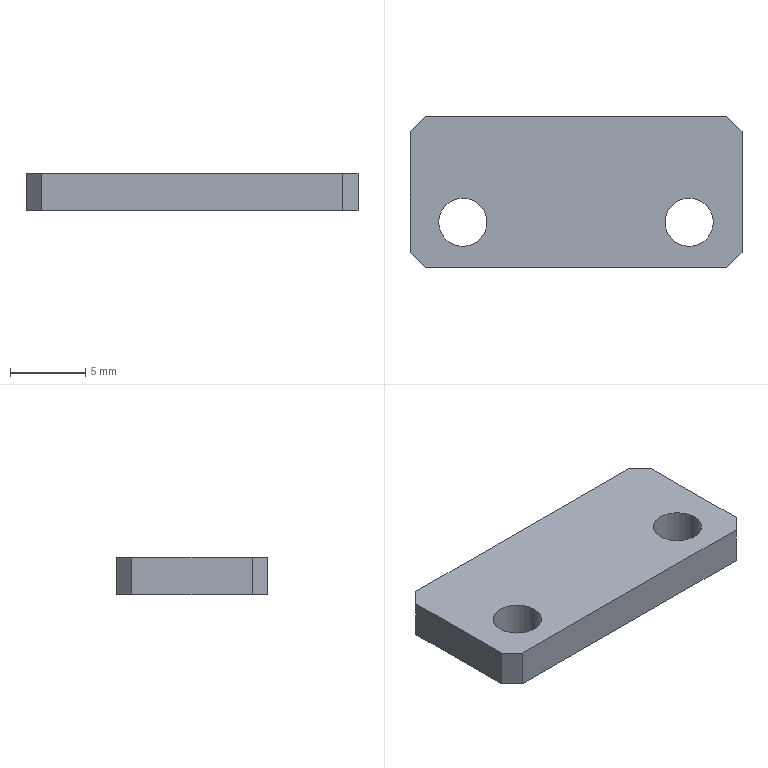Part | NX | features BREP 1 | 1 solid | 14 faces | box 22 x 10 x 2.5 mm | volume 504.788 mm3 | plane 10 | cylinder 4 | commonest cylinder face diameters 3.2 x4
STEP:
#1=CARTESIAN_POINT('',(-697.082,-312.703,0.));
#2=VERTEX_POINT('',#1);
#3=CARTESIAN_POINT('',(-693.882,-312.703,0.));
#4=VERTEX_POINT('',#3);
#5=CARTESIAN_POINT('',(-695.482,-312.703,0.));
#6=DIRECTION('',(0.,0.,1.));
#7=DIRECTION('',(1.,0.,0.));
#8=AXIS2_PLACEMENT_3D('',#5,#6,#7);
#9=CIRCLE('',#8,1.6);
#10=EDGE_CURVE('',#2,#4,#9,.T.);
#11=ORIENTED_EDGE('',*,*,#10,.F.);
#12=CARTESIAN_POINT('',(-697.082,-312.703,2.5));
#13=VERTEX_POINT('',#12);
#14=CARTESIAN_POINT('',(-697.082,-312.703,0.));
#15=DIRECTION('',(0.,0.,1.));
#16=VECTOR('',#15,1000.);
#17=LINE('',#14,#16);
#18=EDGE_CURVE('',#13,#2,#17,.F.);
#19=ORIENTED_EDGE('',*,*,#18,.F.);
#20=CARTESIAN_POINT('',(-693.882,-312.703,2.5));
#21=VERTEX_POINT('',#20);
#22=CARTESIAN_POINT('',(-695.482,-312.703,2.5));
#23=DIRECTION('',(0.,0.,1.));
#24=DIRECTION('',(1.,0.,0.));
#25=AXIS2_PLACEMENT_3D('',#22,#23,#24);
#26=CIRCLE('',#25,1.6);
#27=EDGE_CURVE('',#13,#21,#26,.T.);
#28=ORIENTED_EDGE('',*,*,#27,.T.);
#29=CARTESIAN_POINT('',(-693.882,-312.703,0.));
#30=DIRECTION('',(0.,0.,1.));
#31=VECTOR('',#30,1000.);
#32=LINE('',#29,#31);
#33=EDGE_CURVE('',#21,#4,#32,.F.);
#34=ORIENTED_EDGE('',*,*,#33,.T.);
#35=EDGE_LOOP('',(#11,#19,#28,#34));
#36=FACE_BOUND('',#35,.T.);
#37=CARTESIAN_POINT('',(-695.482,-312.703,0.));
#38=DIRECTION('',(0.,0.,1.));
#39=DIRECTION('',(1.,0.,0.));
#40=AXIS2_PLACEMENT_3D('',#37,#38,#39);
#41=CYLINDRICAL_SURFACE('',#40,1.6);
#42=ADVANCED_FACE('',(#36),#41,.F.);
#43=CARTESIAN_POINT('',(-712.082,-312.703,0.));
#44=VERTEX_POINT('',#43);
#45=CARTESIAN_POINT('',(-708.882,-312.703,0.));
#46=VERTEX_POINT('',#45);
#47=CARTESIAN_POINT('',(-710.482,-312.703,0.));
#48=DIRECTION('',(0.,0.,1.));
#49=DIRECTION('',(1.,0.,0.));
#50=AXIS2_PLACEMENT_3D('',#47,#48,#49);
#51=CIRCLE('',#50,1.6);
#52=EDGE_CURVE('',#44,#46,#51,.T.);
#53=ORIENTED_EDGE('',*,*,#52,.F.);
#54=CARTESIAN_POINT('',(-712.082,-312.703,2.5));
#55=VERTEX_POINT('',#54);
#56=CARTESIAN_POINT('',(-712.082,-312.703,0.));
#57=DIRECTION('',(0.,0.,1.));
#58=VECTOR('',#57,1000.);
#59=LINE('',#56,#58);
#60=EDGE_CURVE('',#55,#44,#59,.F.);
#61=ORIENTED_EDGE('',*,*,#60,.F.);
#62=CARTESIAN_POINT('',(-708.882,-312.703,2.5));
#63=VERTEX_POINT('',#62);
#64=CARTESIAN_POINT('',(-710.482,-312.703,2.5));
#65=DIRECTION('',(0.,0.,1.));
#66=DIRECTION('',(1.,0.,0.));
#67=AXIS2_PLACEMENT_3D('',#64,#65,#66);
#68=CIRCLE('',#67,1.6);
#69=EDGE_CURVE('',#55,#63,#68,.T.);
#70=ORIENTED_EDGE('',*,*,#69,.T.);
#71=CARTESIAN_POINT('',(-708.882,-312.703,0.));
#72=DIRECTION('',(0.,0.,1.));
#73=VECTOR('',#72,1000.);
#74=LINE('',#71,#73);
#75=EDGE_CURVE('',#63,#46,#74,.F.);
#76=ORIENTED_EDGE('',*,*,#75,.T.);
#77=EDGE_LOOP('',(#53,#61,#70,#76));
#78=FACE_BOUND('',#77,.T.);
#79=CARTESIAN_POINT('',(-710.482,-312.703,0.));
#80=DIRECTION('',(0.,0.,1.));
#81=DIRECTION('',(1.,0.,0.));
#82=AXIS2_PLACEMENT_3D('',#79,#80,#81);
#83=CYLINDRICAL_SURFACE('',#82,1.6);
#84=ADVANCED_FACE('',(#78),#83,.F.);
#85=CARTESIAN_POINT('',(-713.982,-306.703,2.5));
#86=VERTEX_POINT('',#85);
#87=CARTESIAN_POINT('',(-713.982,-314.703,2.5));
#88=VERTEX_POINT('',#87);
#89=CARTESIAN_POINT('',(-713.982,-305.703,2.5));
#90=DIRECTION('',(0.,-1.,0.));
#91=VECTOR('',#90,1000.);
#92=LINE('',#89,#91);
#93=EDGE_CURVE('',#86,#88,#92,.T.);
#94=ORIENTED_EDGE('',*,*,#93,.F.);
#95=CARTESIAN_POINT('',(-713.982,-306.703,0.));
#96=VERTEX_POINT('',#95);
#97=CARTESIAN_POINT('',(-713.982,-306.703,2.5));
#98=DIRECTION('',(0.,0.,-1.));
#99=VECTOR('',#98,1000.);
#100=LINE('',#97,#99);
#101=EDGE_CURVE('',#86,#96,#100,.T.);
#102=ORIENTED_EDGE('',*,*,#101,.T.);
#103=CARTESIAN_POINT('',(-713.982,-314.703,0.));
#104=VERTEX_POINT('',#103);
#105=CARTESIAN_POINT('',(-713.982,-305.703,0.));
#106=DIRECTION('',(0.,-1.,0.));
#107=VECTOR('',#106,1000.);
#108=LINE('',#105,#107);
#109=EDGE_CURVE('',#96,#104,#108,.T.);
#110=ORIENTED_EDGE('',*,*,#109,.T.);
#111=CARTESIAN_POINT('',(-713.982,-314.703,2.5));
#112=DIRECTION('',(0.,0.,1.));
#113=VECTOR('',#112,1000.);
#114=LINE('',#111,#113);
#115=EDGE_CURVE('',#104,#88,#114,.T.);
#116=ORIENTED_EDGE('',*,*,#115,.T.);
#117=EDGE_LOOP('',(#94,#102,#110,#116));
#118=FACE_BOUND('',#117,.T.);
#119=CARTESIAN_POINT('',(-713.982,-305.703,2.5));
#120=DIRECTION('',(1.,0.,0.));
#121=DIRECTION('',(0.,1.,0.));
#122=AXIS2_PLACEMENT_3D('',#119,#120,#121);
#123=PLANE('',#122);
#124=ADVANCED_FACE('',(#118),#123,.F.);
#125=CARTESIAN_POINT('',(-712.982,-315.703,0.));
#126=VERTEX_POINT('',#125);
#127=CARTESIAN_POINT('',(-692.982,-315.703,0.));
#128=VERTEX_POINT('',#127);
#129=CARTESIAN_POINT('',(-713.982,-315.703,0.));
#130=DIRECTION('',(1.,0.,0.));
#131=VECTOR('',#130,1000.);
#132=LINE('',#129,#131);
#133=EDGE_CURVE('',#126,#128,#132,.T.);
#134=ORIENTED_EDGE('',*,*,#133,.T.);
#135=CARTESIAN_POINT('',(-692.982,-315.703,2.5));
#136=VERTEX_POINT('',#135);
#137=CARTESIAN_POINT('',(-692.982,-315.703,2.5));
#138=DIRECTION('',(0.,0.,1.));
#139=VECTOR('',#138,1000.);
#140=LINE('',#137,#139);
#141=EDGE_CURVE('',#128,#136,#140,.T.);
#142=ORIENTED_EDGE('',*,*,#141,.T.);
#143=CARTESIAN_POINT('',(-712.982,-315.703,2.5));
#144=VERTEX_POINT('',#143);
#145=CARTESIAN_POINT('',(-713.982,-315.703,2.5));
#146=DIRECTION('',(1.,0.,0.));
#147=VECTOR('',#146,1000.);
#148=LINE('',#145,#147);
#149=EDGE_CURVE('',#144,#136,#148,.T.);
#150=ORIENTED_EDGE('',*,*,#149,.F.);
#151=CARTESIAN_POINT('',(-712.982,-315.703,2.5));
#152=DIRECTION('',(0.,0.,-1.));
#153=VECTOR('',#152,1000.);
#154=LINE('',#151,#153);
#155=EDGE_CURVE('',#144,#126,#154,.T.);
#156=ORIENTED_EDGE('',*,*,#155,.T.);
#157=EDGE_LOOP('',(#134,#142,#150,#156));
#158=FACE_BOUND('',#157,.T.);
#159=CARTESIAN_POINT('',(-713.982,-315.703,2.5));
#160=DIRECTION('',(0.,1.,0.));
#161=DIRECTION('',(1.,0.,0.));
#162=AXIS2_PLACEMENT_3D('',#159,#160,#161);
#163=PLANE('',#162);
#164=ADVANCED_FACE('',(#158),#163,.F.);
#165=CARTESIAN_POINT('',(-691.982,-314.703,0.));
#166=VERTEX_POINT('',#165);
#167=CARTESIAN_POINT('',(-691.982,-306.703,0.));
#168=VERTEX_POINT('',#167);
#169=CARTESIAN_POINT('',(-691.982,-305.703,0.));
#170=DIRECTION('',(0.,1.,0.));
#171=VECTOR('',#170,1000.);
#172=LINE('',#169,#171);
#173=EDGE_CURVE('',#166,#168,#172,.T.);
#174=ORIENTED_EDGE('',*,*,#173,.T.);
#175=CARTESIAN_POINT('',(-691.982,-306.703,2.5));
#176=VERTEX_POINT('',#175);
#177=CARTESIAN_POINT('',(-691.982,-306.703,2.5));
#178=DIRECTION('',(0.,0.,1.));
#179=VECTOR('',#178,1000.);
#180=LINE('',#177,#179);
#181=EDGE_CURVE('',#168,#176,#180,.T.);
#182=ORIENTED_EDGE('',*,*,#181,.T.);
#183=CARTESIAN_POINT('',(-691.982,-314.703,2.5));
#184=VERTEX_POINT('',#183);
#185=CARTESIAN_POINT('',(-691.982,-305.703,2.5));
#186=DIRECTION('',(0.,1.,0.));
#187=VECTOR('',#186,1000.);
#188=LINE('',#185,#187);
#189=EDGE_CURVE('',#184,#176,#188,.T.);
#190=ORIENTED_EDGE('',*,*,#189,.F.);
#191=CARTESIAN_POINT('',(-691.982,-314.703,2.5));
#192=DIRECTION('',(0.,0.,-1.));
#193=VECTOR('',#192,1000.);
#194=LINE('',#191,#193);
#195=EDGE_CURVE('',#184,#166,#194,.T.);
#196=ORIENTED_EDGE('',*,*,#195,.T.);
#197=EDGE_LOOP('',(#174,#182,#190,#196));
#198=FACE_BOUND('',#197,.T.);
#199=CARTESIAN_POINT('',(-691.982,-305.703,2.5));
#200=DIRECTION('',(-1.,0.,0.));
#201=DIRECTION('',(0.,0.,1.));
#202=AXIS2_PLACEMENT_3D('',#199,#200,#201);
#203=PLANE('',#202);
#204=ADVANCED_FACE('',(#198),#203,.F.);
#205=CARTESIAN_POINT('',(-692.982,-305.703,0.));
#206=VERTEX_POINT('',#205);
#207=CARTESIAN_POINT('',(-712.982,-305.703,0.));
#208=VERTEX_POINT('',#207);
#209=CARTESIAN_POINT('',(-713.982,-305.703,0.));
#210=DIRECTION('',(-1.,0.,0.));
#211=VECTOR('',#210,1000.);
#212=LINE('',#209,#211);
#213=EDGE_CURVE('',#206,#208,#212,.T.);
#214=ORIENTED_EDGE('',*,*,#213,.T.);
#215=CARTESIAN_POINT('',(-712.982,-305.703,2.5));
#216=VERTEX_POINT('',#215);
#217=CARTESIAN_POINT('',(-712.982,-305.703,2.5));
#218=DIRECTION('',(0.,0.,1.));
#219=VECTOR('',#218,1000.);
#220=LINE('',#217,#219);
#221=EDGE_CURVE('',#208,#216,#220,.T.);
#222=ORIENTED_EDGE('',*,*,#221,.T.);
#223=CARTESIAN_POINT('',(-692.982,-305.703,2.5));
#224=VERTEX_POINT('',#223);
#225=CARTESIAN_POINT('',(-713.982,-305.703,2.5));
#226=DIRECTION('',(-1.,0.,0.));
#227=VECTOR('',#226,1000.);
#228=LINE('',#225,#227);
#229=EDGE_CURVE('',#224,#216,#228,.T.);
#230=ORIENTED_EDGE('',*,*,#229,.F.);
#231=CARTESIAN_POINT('',(-692.982,-305.703,2.5));
#232=DIRECTION('',(0.,0.,-1.));
#233=VECTOR('',#232,1000.);
#234=LINE('',#231,#233);
#235=EDGE_CURVE('',#224,#206,#234,.T.);
#236=ORIENTED_EDGE('',*,*,#235,.T.);
#237=EDGE_LOOP('',(#214,#222,#230,#236));
#238=FACE_BOUND('',#237,.T.);
#239=CARTESIAN_POINT('',(-713.982,-305.703,2.5));
#240=DIRECTION('',(0.,-1.,0.));
#241=DIRECTION('',(0.,0.,-1.));
#242=AXIS2_PLACEMENT_3D('',#239,#240,#241);
#243=PLANE('',#242);
#244=ADVANCED_FACE('',(#238),#243,.F.);
#245=ORIENTED_EDGE('',*,*,#229,.T.);
#246=CARTESIAN_POINT('',(-718.482,-311.203,2.5));
#247=DIRECTION('',(-0.7071,-0.7071,0.));
#248=VECTOR('',#247,1000.);
#249=LINE('',#246,#248);
#250=EDGE_CURVE('',#216,#86,#249,.T.);
#251=ORIENTED_EDGE('',*,*,#250,.T.);
#252=ORIENTED_EDGE('',*,*,#93,.T.);
#253=CARTESIAN_POINT('',(-713.482,-315.203,2.5));
#254=DIRECTION('',(0.7071,-0.7071,0.));
#255=VECTOR('',#254,1000.);
#256=LINE('',#253,#255);
#257=EDGE_CURVE('',#88,#144,#256,.T.);
#258=ORIENTED_EDGE('',*,*,#257,.T.);
#259=ORIENTED_EDGE('',*,*,#149,.T.);
#260=CARTESIAN_POINT('',(-703.482,-326.203,2.5));
#261=DIRECTION('',(0.7071,0.7071,0.));
#262=VECTOR('',#261,1000.);
#263=LINE('',#260,#262);
#264=EDGE_CURVE('',#136,#184,#263,.T.);
#265=ORIENTED_EDGE('',*,*,#264,.T.);
#266=ORIENTED_EDGE('',*,*,#189,.T.);
#267=CARTESIAN_POINT('',(-698.482,-300.203,2.5));
#268=DIRECTION('',(-0.7071,0.7071,0.));
#269=VECTOR('',#268,1000.);
#270=LINE('',#267,#269);
#271=EDGE_CURVE('',#176,#224,#270,.T.);
#272=ORIENTED_EDGE('',*,*,#271,.T.);
#273=EDGE_LOOP('',(#245,#251,#252,#258,#259,#265,#266,#272));
#274=FACE_BOUND('',#273,.T.);
#275=CARTESIAN_POINT('',(-695.482,-312.703,2.5));
#276=DIRECTION('',(0.,0.,1.));
#277=DIRECTION('',(1.,0.,0.));
#278=AXIS2_PLACEMENT_3D('',#275,#276,#277);
#279=CIRCLE('',#278,1.6);
#280=EDGE_CURVE('',#21,#13,#279,.T.);
#281=ORIENTED_EDGE('',*,*,#280,.F.);
#282=ORIENTED_EDGE('',*,*,#27,.F.);
#283=EDGE_LOOP('',(#281,#282));
#284=FACE_BOUND('',#283,.T.);
#285=CARTESIAN_POINT('',(-710.482,-312.703,2.5));
#286=DIRECTION('',(0.,0.,1.));
#287=DIRECTION('',(1.,0.,0.));
#288=AXIS2_PLACEMENT_3D('',#285,#286,#287);
#289=CIRCLE('',#288,1.6);
#290=EDGE_CURVE('',#63,#55,#289,.T.);
#291=ORIENTED_EDGE('',*,*,#290,.F.);
#292=ORIENTED_EDGE('',*,*,#69,.F.);
#293=EDGE_LOOP('',(#291,#292));
#294=FACE_BOUND('',#293,.T.);
#295=CARTESIAN_POINT('',(-713.982,-315.703,2.5));
#296=DIRECTION('',(0.,0.,1.));
#297=DIRECTION('',(1.,0.,0.));
#298=AXIS2_PLACEMENT_3D('',#295,#296,#297);
#299=PLANE('',#298);
#300=ADVANCED_FACE('',(#274,#284,#294),#299,.T.);
#301=ORIENTED_EDGE('',*,*,#109,.F.);
#302=CARTESIAN_POINT('',(-713.982,-306.703,0.));
#303=DIRECTION('',(0.7071,0.7071,0.));
#304=VECTOR('',#303,1000.);
#305=LINE('',#302,#304);
#306=EDGE_CURVE('',#96,#208,#305,.T.);
#307=ORIENTED_EDGE('',*,*,#306,.T.);
#308=ORIENTED_EDGE('',*,*,#213,.F.);
#309=CARTESIAN_POINT('',(-692.982,-305.703,0.));
#310=DIRECTION('',(0.7071,-0.7071,0.));
#311=VECTOR('',#310,1000.);
#312=LINE('',#309,#311);
#313=EDGE_CURVE('',#206,#168,#312,.T.);
#314=ORIENTED_EDGE('',*,*,#313,.T.);
#315=ORIENTED_EDGE('',*,*,#173,.F.);
#316=CARTESIAN_POINT('',(-691.982,-314.703,0.));
#317=DIRECTION('',(-0.7071,-0.7071,0.));
#318=VECTOR('',#317,1000.);
#319=LINE('',#316,#318);
#320=EDGE_CURVE('',#166,#128,#319,.T.);
#321=ORIENTED_EDGE('',*,*,#320,.T.);
#322=ORIENTED_EDGE('',*,*,#133,.F.);
#323=CARTESIAN_POINT('',(-712.982,-315.703,0.));
#324=DIRECTION('',(-0.7071,0.7071,0.));
#325=VECTOR('',#324,1000.);
#326=LINE('',#323,#325);
#327=EDGE_CURVE('',#126,#104,#326,.T.);
#328=ORIENTED_EDGE('',*,*,#327,.T.);
#329=EDGE_LOOP('',(#301,#307,#308,#314,#315,#321,#322,#328));
#330=FACE_BOUND('',#329,.T.);
#331=CARTESIAN_POINT('',(-695.482,-312.703,0.));
#332=DIRECTION('',(0.,0.,1.));
#333=DIRECTION('',(1.,0.,0.));
#334=AXIS2_PLACEMENT_3D('',#331,#332,#333);
#335=CIRCLE('',#334,1.6);
#336=EDGE_CURVE('',#4,#2,#335,.T.);
#337=ORIENTED_EDGE('',*,*,#336,.T.);
#338=ORIENTED_EDGE('',*,*,#10,.T.);
#339=EDGE_LOOP('',(#337,#338));
#340=FACE_BOUND('',#339,.T.);
#341=CARTESIAN_POINT('',(-710.482,-312.703,0.));
#342=DIRECTION('',(0.,0.,1.));
#343=DIRECTION('',(1.,0.,0.));
#344=AXIS2_PLACEMENT_3D('',#341,#342,#343);
#345=CIRCLE('',#344,1.6);
#346=EDGE_CURVE('',#46,#44,#345,.T.);
#347=ORIENTED_EDGE('',*,*,#346,.T.);
#348=ORIENTED_EDGE('',*,*,#52,.T.);
#349=EDGE_LOOP('',(#347,#348));
#350=FACE_BOUND('',#349,.T.);
#351=CARTESIAN_POINT('',(-713.982,-315.703,0.));
#352=DIRECTION('',(0.,0.,1.));
#353=DIRECTION('',(1.,0.,0.));
#354=AXIS2_PLACEMENT_3D('',#351,#352,#353);
#355=PLANE('',#354);
#356=ADVANCED_FACE('',(#330,#340,#350),#355,.F.);
#357=ORIENTED_EDGE('',*,*,#60,.T.);
#358=ORIENTED_EDGE('',*,*,#346,.F.);
#359=ORIENTED_EDGE('',*,*,#75,.F.);
#360=ORIENTED_EDGE('',*,*,#290,.T.);
#361=EDGE_LOOP('',(#357,#358,#359,#360));
#362=FACE_BOUND('',#361,.T.);
#363=CARTESIAN_POINT('',(-710.482,-312.703,0.));
#364=DIRECTION('',(0.,0.,1.));
#365=DIRECTION('',(1.,0.,0.));
#366=AXIS2_PLACEMENT_3D('',#363,#364,#365);
#367=CYLINDRICAL_SURFACE('',#366,1.6);
#368=ADVANCED_FACE('',(#362),#367,.F.);
#369=ORIENTED_EDGE('',*,*,#18,.T.);
#370=ORIENTED_EDGE('',*,*,#336,.F.);
#371=ORIENTED_EDGE('',*,*,#33,.F.);
#372=ORIENTED_EDGE('',*,*,#280,.T.);
#373=EDGE_LOOP('',(#369,#370,#371,#372));
#374=FACE_BOUND('',#373,.T.);
#375=CARTESIAN_POINT('',(-695.482,-312.703,0.));
#376=DIRECTION('',(0.,0.,1.));
#377=DIRECTION('',(1.,0.,0.));
#378=AXIS2_PLACEMENT_3D('',#375,#376,#377);
#379=CYLINDRICAL_SURFACE('',#378,1.6);
#380=ADVANCED_FACE('',(#374),#379,.F.);
#381=ORIENTED_EDGE('',*,*,#250,.F.);
#382=ORIENTED_EDGE('',*,*,#221,.F.);
#383=ORIENTED_EDGE('',*,*,#306,.F.);
#384=ORIENTED_EDGE('',*,*,#101,.F.);
#385=EDGE_LOOP('',(#381,#382,#383,#384));
#386=FACE_BOUND('',#385,.T.);
#387=CARTESIAN_POINT('',(-713.982,-306.703,2.5));
#388=DIRECTION('',(0.7071,-0.7071,0.));
#389=DIRECTION('',(0.,0.,-1.));
#390=AXIS2_PLACEMENT_3D('',#387,#388,#389);
#391=PLANE('',#390);
#392=ADVANCED_FACE('',(#386),#391,.F.);
#393=ORIENTED_EDGE('',*,*,#271,.F.);
#394=ORIENTED_EDGE('',*,*,#181,.F.);
#395=ORIENTED_EDGE('',*,*,#313,.F.);
#396=ORIENTED_EDGE('',*,*,#235,.F.);
#397=EDGE_LOOP('',(#393,#394,#395,#396));
#398=FACE_BOUND('',#397,.T.);
#399=CARTESIAN_POINT('',(-692.982,-305.703,2.5));
#400=DIRECTION('',(-0.7071,-0.7071,0.));
#401=DIRECTION('',(-0.7071,0.7071,0.));
#402=AXIS2_PLACEMENT_3D('',#399,#400,#401);
#403=PLANE('',#402);
#404=ADVANCED_FACE('',(#398),#403,.F.);
#405=ORIENTED_EDGE('',*,*,#264,.F.);
#406=ORIENTED_EDGE('',*,*,#141,.F.);
#407=ORIENTED_EDGE('',*,*,#320,.F.);
#408=ORIENTED_EDGE('',*,*,#195,.F.);
#409=EDGE_LOOP('',(#405,#406,#407,#408));
#410=FACE_BOUND('',#409,.T.);
#411=CARTESIAN_POINT('',(-691.982,-314.703,2.5));
#412=DIRECTION('',(-0.7071,0.7071,0.));
#413=DIRECTION('',(0.,0.,1.));
#414=AXIS2_PLACEMENT_3D('',#411,#412,#413);
#415=PLANE('',#414);
#416=ADVANCED_FACE('',(#410),#415,.F.);
#417=ORIENTED_EDGE('',*,*,#257,.F.);
#418=ORIENTED_EDGE('',*,*,#115,.F.);
#419=ORIENTED_EDGE('',*,*,#327,.F.);
#420=ORIENTED_EDGE('',*,*,#155,.F.);
#421=EDGE_LOOP('',(#417,#418,#419,#420));
#422=FACE_BOUND('',#421,.T.);
#423=CARTESIAN_POINT('',(-712.982,-315.703,2.5));
#424=DIRECTION('',(0.7071,0.7071,0.));
#425=DIRECTION('',(0.,0.,-1.));
#426=AXIS2_PLACEMENT_3D('',#423,#424,#425);
#427=PLANE('',#426);
#428=ADVANCED_FACE('',(#422),#427,.F.);
#429=CLOSED_SHELL('',(#42,#84,#124,#164,#204,#244,#300,#356,#368,#380,#392,#404,#416,#428));
#430=MANIFOLD_SOLID_BREP('',#429);
#431=(LENGTH_UNIT()NAMED_UNIT(*)SI_UNIT(.MILLI.,.METRE.));
#432=UNCERTAINTY_MEASURE_WITH_UNIT(LENGTH_MEASURE(0.00001),#431,'','');
#433=(NAMED_UNIT(*)PLANE_ANGLE_UNIT()SI_UNIT($,.RADIAN.));
#434=(NAMED_UNIT(*)SI_UNIT($,.STERADIAN.)SOLID_ANGLE_UNIT());
#435=(GEOMETRIC_REPRESENTATION_CONTEXT(3)GLOBAL_UNCERTAINTY_ASSIGNED_CONTEXT((#432))GLOBAL_UNIT_ASSIGNED_CONTEXT((#431,#433,#434))REPRESENTATION_CONTEXT('',''));
#436=ADVANCED_BREP_SHAPE_REPRESENTATION('',(#430),#435);